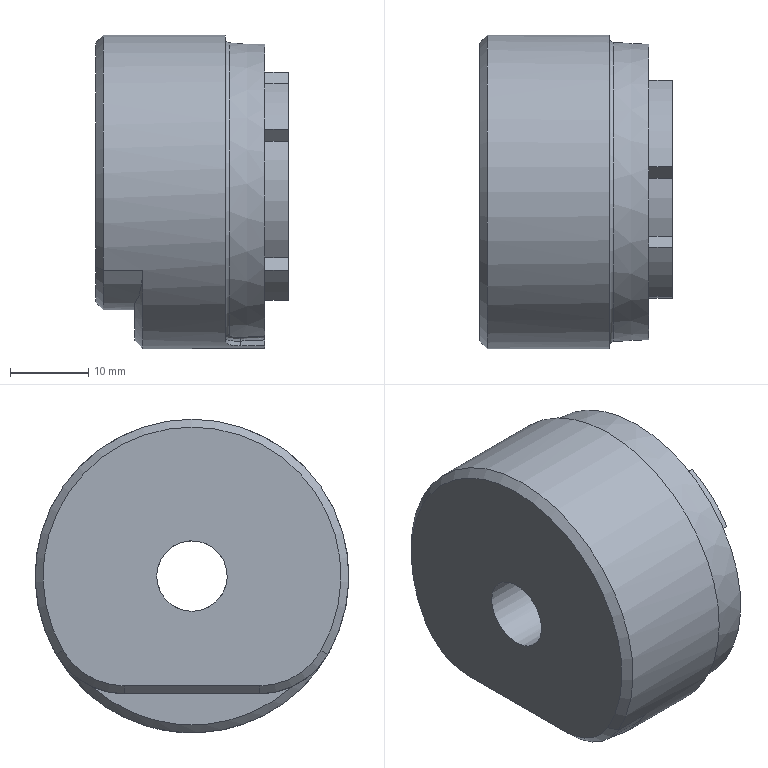Part | STEP file | solid 240 | 1 solid | 43 faces | box 24.594 x 40 x 40 mm | volume 25514 mm3 | plane 18 | cylinder 15 | cone 5 | spline 4 | torus 1 | commonest cylinder face diameters 27.135 x4 31.155 x4 4.02 x2 20 x2 9 x1 14 x1